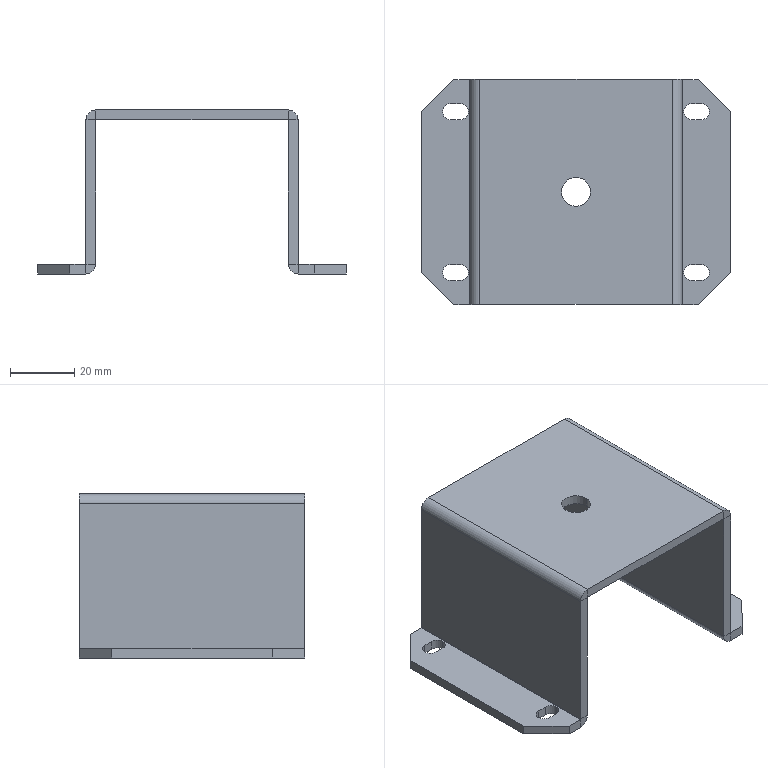Part | SolidWorks | features EdgeFlange 3, ICE 2, Chamfer 1, FlatPattern 1, SMBaseFlange 1, SheetMetal 1 | 1 solid | 64 faces | box 96 x 70 x 51 mm | volume 38537 mm3 | plane 42 | cylinder 22 | commonest cylinder face diameters 5 x12 0.2 x4 6.2 x4 9 x2